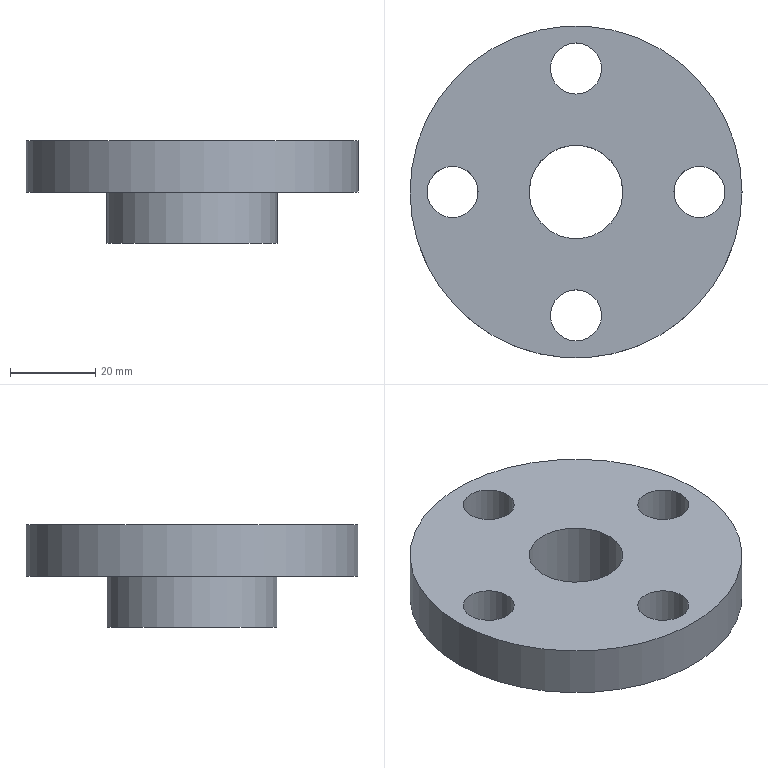NC program | NX | posted with a generic post | part box 78 x 78 x 24 mm
Whole program:
N10 G17 G21 G94 G90
(DRILLING , TOOL : ZXZ)
N12 T01 M6
N14 G54
N16 G17 G0 G90 X29. Y0. S3000 M3
N18 G43 Z30. H1
N20 G94 G81 G98 Z-1. F200. R3.
N22 X0. Y29.
N24 X-29. Y0.
N26 X0. Y-29.
N28 G80
N30 G0 X0. Y-29. Z30.
N32 M5
(DRILLING_COPY , TOOL : 12.0ZT)
N34 T02 M6
N36 G54
N38 G17 G0 G90 X29. Y0. S800 M3
N40 G43 Z30. H2
N42 G94 G83 G98 Z-17.105 F150. Q2. R3.
N44 X0. Y29.
N46 X-29. Y0.
N48 X0. Y-29.
N50 G80
N52 G0 X0. Y-29. Z30.
N54 M5
(ZLEVEL_PROFILE_1_COPY_1 , TOOL : D6A45)
N56 T07 M6
N58 G54
N60 G17 G0 G90 X1.136 Y32.756 S7500 M3
N62 G43 Z30. H7
N64 Z0.
N66 G94 G1 Z-1. F1000.
N68 X0.52 Y33.824
N70 G3 X0. Y34.124 R0.6
N72 X-5.124 Y29. R5.124
N74 X0. Y34.124 R-5.124
N76 X-0.52 Y33.824 R0.6
N78 G1 X-1.136 Y32.756
N80 Z0.
N82 G0 Z30.
N84 X32.756 Y-1.136
N86 Z0.
N88 G1 Z-1.
N90 X33.824 Y-0.52
N92 G3 X34.124 Y0. R0.6
N94 X29. Y5.124 R5.124
N96 X34.124 Y0. R-5.124
N98 X33.824 Y0.52 R0.6
N100 G1 X32.756 Y1.136
N102 Z0.
N104 G0 Z30.
N106 X-32.756
N108 Z0.
N110 G1 Z-1.
N112 X-33.824 Y0.52
N114 G3 X-34.124 Y0. R0.6
N116 X-29. Y-5.124 R5.124
N118 X-34.124 Y0. R-5.124
N120 X-33.824 Y-0.52 R0.6
N122 G1 X-32.756 Y-1.136
N124 Z0.
N126 G0 Z30.
N128 X-1.136 Y-32.756
N130 Z0.
N132 G1 Z-1.
N134 X-0.52 Y-33.824
N136 G3 X0. Y-34.124 R0.6
N138 X5.124 Y-29. R5.124
N140 X0. Y-34.124 R-5.124
N142 X0.52 Y-33.824 R0.6
N144 G1 X1.136 Y-32.756
N146 Z0.
N148 G0 Z30.
N150 M5
N152 M2